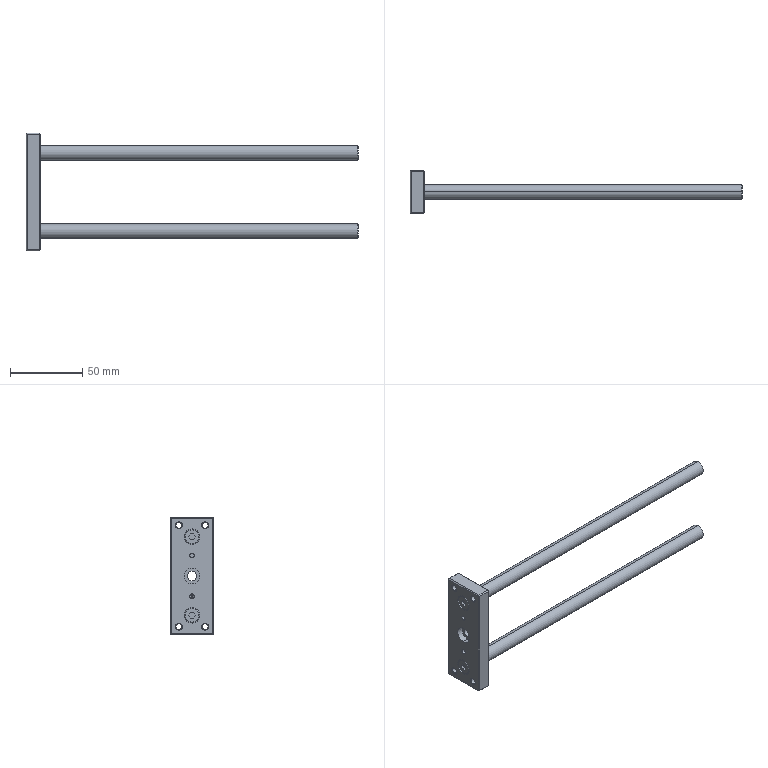Part | STEP file | TC-L-20x125_125fp_HI | 1 solid | 101 faces | box 229 x 30 x 81 mm | volume 57198 mm3 | plane 44 | cylinder 31 | cone 22 | torus 4 | commonest cylinder face diameters 4.134 x8 3 x7 11 x6 10 x4 10.5 x4 6.4 x2